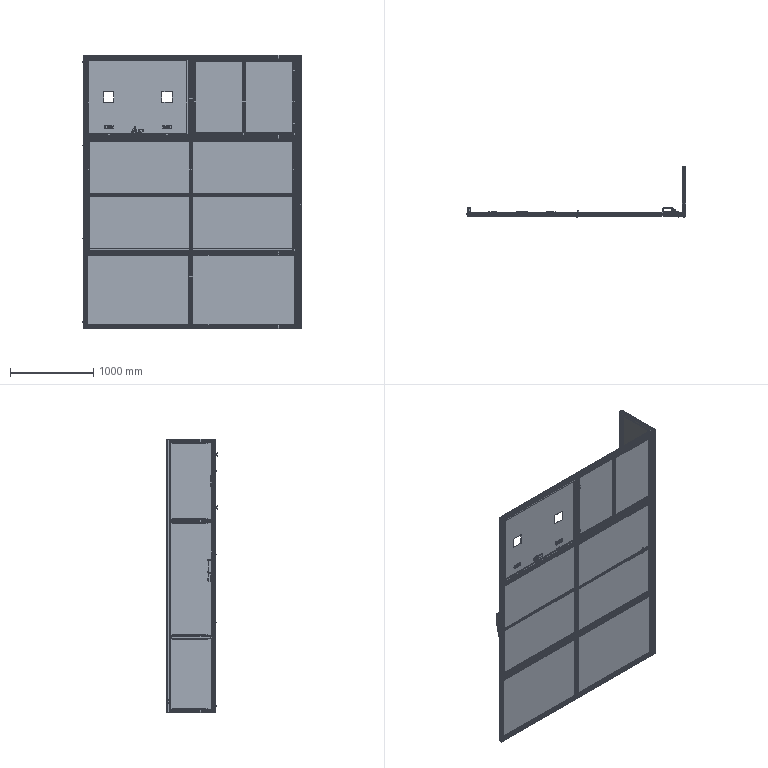Part | SolidWorks | 228 solids | 11616 faces | volume 65477431 mm3 | plane 7099 | cylinder 3318 | cone 889 | spline 290 | torus 20 | commonest cylinder face diameters 5 x384 6.8 x338 1 x274 2 x270 11 x268 6 x138